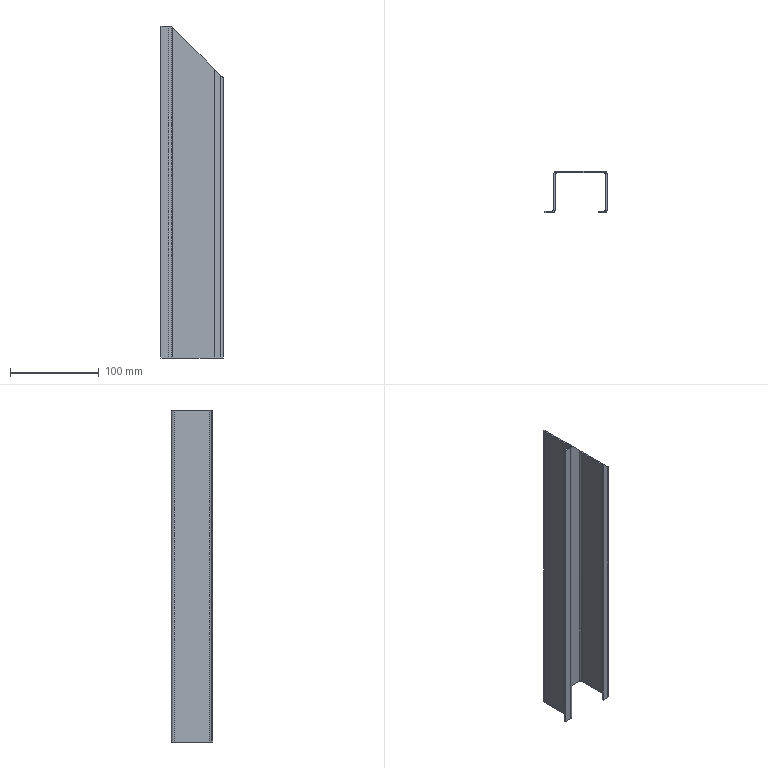Part | STEP file | 750078417 | 1 solid | 28 faces | box 70 x 46.5 x 374 mm | volume 85341 mm3 | plane 17 | cylinder 8 | spline 3 | commonest cylinder face diameters 3 x4 6 x4
STEP:
#1=CARTESIAN_POINT('',(-14.5,45.,318.5));
#2=VERTEX_POINT('',#1);
#3=CARTESIAN_POINT('',(-14.5,45.,0.));
#4=VERTEX_POINT('',#3);
#5=CARTESIAN_POINT('',(-14.5,45.,0.));
#6=DIRECTION('',(0.,0.,-1.));
#7=VECTOR('',#6,1000.);
#8=LINE('',#5,#7);
#9=EDGE_CURVE('',#2,#4,#8,.T.);
#10=ORIENTED_EDGE('',*,*,#9,.T.);
#11=CARTESIAN_POINT('',(-68.5,45.,0.));
#12=VERTEX_POINT('',#11);
#13=CARTESIAN_POINT('',(-11.5,45.,0.));
#14=DIRECTION('',(-1.,0.,0.));
#15=VECTOR('',#14,1000.);
#16=LINE('',#13,#15);
#17=EDGE_CURVE('',#4,#12,#16,.T.);
#18=ORIENTED_EDGE('',*,*,#17,.T.);
#19=CARTESIAN_POINT('',(-68.5,45.,372.5));
#20=VERTEX_POINT('',#19);
#21=CARTESIAN_POINT('',(-68.5,45.,0.));
#22=DIRECTION('',(0.,0.,1.));
#23=VECTOR('',#22,1000.);
#24=LINE('',#21,#23);
#25=EDGE_CURVE('',#12,#20,#24,.T.);
#26=ORIENTED_EDGE('',*,*,#25,.T.);
#27=CARTESIAN_POINT('',(-68.5,45.,372.5));
#28=DIRECTION('',(0.7071,0.,-0.7071));
#29=VECTOR('',#28,1000.);
#30=LINE('',#27,#29);
#31=EDGE_CURVE('',#20,#2,#30,.T.);
#32=ORIENTED_EDGE('',*,*,#31,.T.);
#33=EDGE_LOOP('',(#10,#18,#26,#32));
#34=FACE_OUTER_BOUND('',#33,.T.);
#35=CARTESIAN_POINT('',(-11.5,45.,0.));
#36=DIRECTION('',(0.,1.,0.));
#37=DIRECTION('',(-1.,0.,0.));
#38=AXIS2_PLACEMENT_3D('',#35,#36,#37);
#39=PLANE('',#38);
#40=ADVANCED_FACE('',(#34),#39,.T.);
#41=CARTESIAN_POINT('',(-14.5,-1.5,0.));
#42=VERTEX_POINT('',#41);
#43=CARTESIAN_POINT('',(-21.5,-1.5,0.));
#44=VERTEX_POINT('',#43);
#45=CARTESIAN_POINT('',(-21.5,-1.5,0.));
#46=DIRECTION('',(-1.,0.,0.));
#47=VECTOR('',#46,1000.);
#48=LINE('',#45,#47);
#49=EDGE_CURVE('',#42,#44,#48,.T.);
#50=ORIENTED_EDGE('',*,*,#49,.T.);
#51=CARTESIAN_POINT('',(-21.5,0.,0.));
#52=VERTEX_POINT('',#51);
#53=CARTESIAN_POINT('',(-21.5,-1.5,0.));
#54=DIRECTION('',(0.,1.,0.));
#55=VECTOR('',#54,1000.);
#56=LINE('',#53,#55);
#57=EDGE_CURVE('',#44,#52,#56,.T.);
#58=ORIENTED_EDGE('',*,*,#57,.T.);
#59=CARTESIAN_POINT('',(-14.5,0.,0.));
#60=VERTEX_POINT('',#59);
#61=CARTESIAN_POINT('',(-21.5,0.,0.));
#62=DIRECTION('',(1.,0.,0.));
#63=VECTOR('',#62,1000.);
#64=LINE('',#61,#63);
#65=EDGE_CURVE('',#52,#60,#64,.T.);
#66=ORIENTED_EDGE('',*,*,#65,.T.);
#67=CARTESIAN_POINT('',(-13.,1.5,0.));
#68=VERTEX_POINT('',#67);
#69=CARTESIAN_POINT('',(-14.5,1.5,0.));
#70=DIRECTION('',(0.,0.,1.));
#71=DIRECTION('',(1.,0.,0.));
#72=AXIS2_PLACEMENT_3D('',#69,#70,#71);
#73=CIRCLE('',#72,1.5);
#74=EDGE_CURVE('',#60,#68,#73,.T.);
#75=ORIENTED_EDGE('',*,*,#74,.T.);
#76=CARTESIAN_POINT('',(-13.,42.,0.));
#77=VERTEX_POINT('',#76);
#78=CARTESIAN_POINT('',(-13.,-1.5,0.));
#79=DIRECTION('',(0.,1.,0.));
#80=VECTOR('',#79,1000.);
#81=LINE('',#78,#80);
#82=EDGE_CURVE('',#68,#77,#81,.T.);
#83=ORIENTED_EDGE('',*,*,#82,.T.);
#84=CARTESIAN_POINT('',(-14.5,43.5,0.));
#85=VERTEX_POINT('',#84);
#86=CARTESIAN_POINT('',(-14.5,42.,0.));
#87=DIRECTION('',(0.,0.,1.));
#88=DIRECTION('',(1.,0.,0.));
#89=AXIS2_PLACEMENT_3D('',#86,#87,#88);
#90=CIRCLE('',#89,1.5);
#91=EDGE_CURVE('',#77,#85,#90,.T.);
#92=ORIENTED_EDGE('',*,*,#91,.T.);
#93=CARTESIAN_POINT('',(-68.5,43.5,0.));
#94=VERTEX_POINT('',#93);
#95=CARTESIAN_POINT('',(-21.5,43.5,0.));
#96=DIRECTION('',(-1.,0.,0.));
#97=VECTOR('',#96,1000.);
#98=LINE('',#95,#97);
#99=EDGE_CURVE('',#85,#94,#98,.T.);
#100=ORIENTED_EDGE('',*,*,#99,.T.);
#101=CARTESIAN_POINT('',(-70.,42.,0.));
#102=VERTEX_POINT('',#101);
#103=CARTESIAN_POINT('',(-68.5,42.,0.));
#104=DIRECTION('',(0.,0.,1.));
#105=DIRECTION('',(1.,0.,0.));
#106=AXIS2_PLACEMENT_3D('',#103,#104,#105);
#107=CIRCLE('',#106,1.5);
#108=EDGE_CURVE('',#94,#102,#107,.T.);
#109=ORIENTED_EDGE('',*,*,#108,.T.);
#110=CARTESIAN_POINT('',(-70.,1.5,0.));
#111=VERTEX_POINT('',#110);
#112=CARTESIAN_POINT('',(-70.,-1.5,0.));
#113=DIRECTION('',(0.,-1.,0.));
#114=VECTOR('',#113,1000.);
#115=LINE('',#112,#114);
#116=EDGE_CURVE('',#102,#111,#115,.T.);
#117=ORIENTED_EDGE('',*,*,#116,.T.);
#118=CARTESIAN_POINT('',(-73.,-1.5,0.));
#119=VERTEX_POINT('',#118);
#120=CARTESIAN_POINT('',(-73.,1.5,0.));
#121=DIRECTION('',(0.,0.,-1.));
#122=DIRECTION('',(1.,0.,0.));
#123=AXIS2_PLACEMENT_3D('',#120,#121,#122);
#124=CIRCLE('',#123,3.);
#125=EDGE_CURVE('',#111,#119,#124,.T.);
#126=ORIENTED_EDGE('',*,*,#125,.T.);
#127=CARTESIAN_POINT('',(-81.5,-1.5,0.));
#128=VERTEX_POINT('',#127);
#129=CARTESIAN_POINT('',(-21.5,-1.5,0.));
#130=DIRECTION('',(-1.,0.,0.));
#131=VECTOR('',#130,1000.);
#132=LINE('',#129,#131);
#133=EDGE_CURVE('',#119,#128,#132,.T.);
#134=ORIENTED_EDGE('',*,*,#133,.T.);
#135=CARTESIAN_POINT('',(-81.5,0.,0.));
#136=VERTEX_POINT('',#135);
#137=CARTESIAN_POINT('',(-81.5,0.,0.));
#138=DIRECTION('',(0.,-1.,0.));
#139=VECTOR('',#138,1000.);
#140=LINE('',#137,#139);
#141=EDGE_CURVE('',#136,#128,#140,.T.);
#142=ORIENTED_EDGE('',*,*,#141,.F.);
#143=CARTESIAN_POINT('',(-73.,0.,0.));
#144=VERTEX_POINT('',#143);
#145=CARTESIAN_POINT('',(-21.5,0.,0.));
#146=DIRECTION('',(1.,0.,0.));
#147=VECTOR('',#146,1000.);
#148=LINE('',#145,#147);
#149=EDGE_CURVE('',#136,#144,#148,.T.);
#150=ORIENTED_EDGE('',*,*,#149,.T.);
#151=CARTESIAN_POINT('',(-71.5,1.5,0.));
#152=VERTEX_POINT('',#151);
#153=CARTESIAN_POINT('',(-73.,1.5,0.));
#154=DIRECTION('',(0.,0.,1.));
#155=DIRECTION('',(1.,0.,0.));
#156=AXIS2_PLACEMENT_3D('',#153,#154,#155);
#157=CIRCLE('',#156,1.5);
#158=EDGE_CURVE('',#144,#152,#157,.T.);
#159=ORIENTED_EDGE('',*,*,#158,.T.);
#160=CARTESIAN_POINT('',(-71.5,42.,0.));
#161=VERTEX_POINT('',#160);
#162=CARTESIAN_POINT('',(-71.5,-1.5,0.));
#163=DIRECTION('',(0.,1.,0.));
#164=VECTOR('',#163,1000.);
#165=LINE('',#162,#164);
#166=EDGE_CURVE('',#152,#161,#165,.T.);
#167=ORIENTED_EDGE('',*,*,#166,.T.);
#168=CARTESIAN_POINT('',(-68.5,42.,0.));
#169=DIRECTION('',(0.,0.,-1.));
#170=DIRECTION('',(1.,0.,0.));
#171=AXIS2_PLACEMENT_3D('',#168,#169,#170);
#172=CIRCLE('',#171,3.);
#173=EDGE_CURVE('',#161,#12,#172,.T.);
#174=ORIENTED_EDGE('',*,*,#173,.T.);
#175=ORIENTED_EDGE('',*,*,#17,.F.);
#176=CARTESIAN_POINT('',(-11.5,42.,0.));
#177=VERTEX_POINT('',#176);
#178=CARTESIAN_POINT('',(-14.5,42.,0.));
#179=DIRECTION('',(0.,0.,-1.));
#180=DIRECTION('',(1.,0.,0.));
#181=AXIS2_PLACEMENT_3D('',#178,#179,#180);
#182=CIRCLE('',#181,3.);
#183=EDGE_CURVE('',#4,#177,#182,.T.);
#184=ORIENTED_EDGE('',*,*,#183,.T.);
#185=CARTESIAN_POINT('',(-11.5,1.5,0.));
#186=VERTEX_POINT('',#185);
#187=CARTESIAN_POINT('',(-11.5,-1.5,0.));
#188=DIRECTION('',(0.,-1.,0.));
#189=VECTOR('',#188,1000.);
#190=LINE('',#187,#189);
#191=EDGE_CURVE('',#177,#186,#190,.T.);
#192=ORIENTED_EDGE('',*,*,#191,.T.);
#193=CARTESIAN_POINT('',(-14.5,1.5,0.));
#194=DIRECTION('',(0.,0.,-1.));
#195=DIRECTION('',(1.,0.,0.));
#196=AXIS2_PLACEMENT_3D('',#193,#194,#195);
#197=CIRCLE('',#196,3.);
#198=EDGE_CURVE('',#186,#42,#197,.T.);
#199=ORIENTED_EDGE('',*,*,#198,.T.);
#200=EDGE_LOOP('',(#50,#58,#66,#75,#83,#92,#100,#109,#117,#126,#134,#142,#150,#159,#167,#174,#175,#184,#192,#199));
#201=FACE_OUTER_BOUND('',#200,.T.);
#202=CARTESIAN_POINT('',(-21.5,-1.5,0.));
#203=DIRECTION('',(0.,0.,-1.));
#204=DIRECTION('',(-1.,0.,0.));
#205=AXIS2_PLACEMENT_3D('',#202,#203,#204);
#206=PLANE('',#205);
#207=ADVANCED_FACE('',(#201),#206,.T.);
#208=CARTESIAN_POINT('',(-11.5,42.,315.5));
#209=VERTEX_POINT('',#208);
#210=CARTESIAN_POINT('',(-11.5,42.,0.));
#211=DIRECTION('',(0.,0.,-1.));
#212=VECTOR('',#211,1000.);
#213=LINE('',#210,#212);
#214=EDGE_CURVE('',#209,#177,#213,.T.);
#215=ORIENTED_EDGE('',*,*,#214,.T.);
#216=ORIENTED_EDGE('',*,*,#183,.F.);
#217=ORIENTED_EDGE('',*,*,#9,.F.);
#218=CARTESIAN_POINT('',(-14.5,45.,318.5));
#219=CARTESIAN_POINT('',(-12.5,45.,316.5));
#220=CARTESIAN_POINT('',(-11.5,43.5,315.5));
#221=CARTESIAN_POINT('',(-11.5,42.,315.5));
#222=(BOUNDED_CURVE()B_SPLINE_CURVE(3,(#218,#219,#220,#221),.UNSPECIFIED.,.F.,.T.)B_SPLINE_CURVE_WITH_KNOTS((4,4),(0.,0.005675),.UNSPECIFIED.)CURVE()GEOMETRIC_REPRESENTATION_ITEM()RATIONAL_B_SPLINE_CURVE((0.5,0.5,0.6667,1.))REPRESENTATION_ITEM(''));
#223=EDGE_CURVE('',#2,#209,#222,.T.);
#224=ORIENTED_EDGE('',*,*,#223,.T.);
#225=EDGE_LOOP('',(#215,#216,#217,#224));
#226=FACE_OUTER_BOUND('',#225,.T.);
#227=CARTESIAN_POINT('',(-14.5,42.,0.));
#228=DIRECTION('',(0.,0.,1.));
#229=DIRECTION('',(1.,0.,0.));
#230=AXIS2_PLACEMENT_3D('',#227,#228,#229);
#231=CYLINDRICAL_SURFACE('',#230,3.);
#232=ADVANCED_FACE('',(#226),#231,.T.);
#233=CARTESIAN_POINT('',(-68.5,43.5,372.5));
#234=VERTEX_POINT('',#233);
#235=CARTESIAN_POINT('',(-68.5,44.25,372.5));
#236=DIRECTION('',(0.,-1.,0.));
#237=VECTOR('',#236,1000.);
#238=LINE('',#235,#237);
#239=EDGE_CURVE('',#20,#234,#238,.T.);
#240=ORIENTED_EDGE('',*,*,#239,.T.);
#241=CARTESIAN_POINT('',(-14.5,43.5,318.5));
#242=VERTEX_POINT('',#241);
#243=CARTESIAN_POINT('',(146.25,43.5,157.75));
#244=DIRECTION('',(0.7071,0.,-0.7071));
#245=VECTOR('',#244,1000.);
#246=LINE('',#243,#245);
#247=EDGE_CURVE('',#234,#242,#246,.T.);
#248=ORIENTED_EDGE('',*,*,#247,.T.);
#249=CARTESIAN_POINT('',(-14.5,45.,318.5));
#250=DIRECTION('',(0.,1.,0.));
#251=VECTOR('',#250,1000.);
#252=LINE('',#249,#251);
#253=EDGE_CURVE('',#242,#2,#252,.T.);
#254=ORIENTED_EDGE('',*,*,#253,.T.);
#255=ORIENTED_EDGE('',*,*,#31,.F.);
#256=EDGE_LOOP('',(#240,#248,#254,#255));
#257=FACE_OUTER_BOUND('',#256,.T.);
#258=CARTESIAN_POINT('',(146.25,45.,157.75));
#259=DIRECTION('',(0.7071,0.,0.7071));
#260=DIRECTION('',(0.7071,0.,-0.7071));
#261=AXIS2_PLACEMENT_3D('',#258,#259,#260);
#262=PLANE('',#261);
#263=ADVANCED_FACE('',(#257),#262,.T.);
#264=ORIENTED_EDGE('',*,*,#25,.F.);
#265=ORIENTED_EDGE('',*,*,#173,.F.);
#266=CARTESIAN_POINT('',(-71.5,42.,374.));
#267=VERTEX_POINT('',#266);
#268=CARTESIAN_POINT('',(-71.5,42.,0.));
#269=DIRECTION('',(0.,0.,1.));
#270=VECTOR('',#269,1000.);
#271=LINE('',#268,#270);
#272=EDGE_CURVE('',#161,#267,#271,.T.);
#273=ORIENTED_EDGE('',*,*,#272,.T.);
#274=CARTESIAN_POINT('',(-71.5,42.,374.));
#275=CARTESIAN_POINT('',(-71.5,43.5,374.));
#276=CARTESIAN_POINT('',(-70.5,45.,373.5));
#277=CARTESIAN_POINT('',(-68.5,45.,372.5));
#278=(BOUNDED_CURVE()B_SPLINE_CURVE(3,(#274,#275,#276,#277),.UNSPECIFIED.,.F.,.F.)B_SPLINE_CURVE_WITH_KNOTS((4,4),(0.,0.00497),.UNSPECIFIED.)CURVE()GEOMETRIC_REPRESENTATION_ITEM()RATIONAL_B_SPLINE_CURVE((1.,0.6667,0.5,0.5))REPRESENTATION_ITEM(''));
#279=EDGE_CURVE('',#267,#20,#278,.T.);
#280=ORIENTED_EDGE('',*,*,#279,.T.);
#281=EDGE_LOOP('',(#264,#265,#273,#280));
#282=FACE_OUTER_BOUND('',#281,.T.);
#283=CARTESIAN_POINT('',(-68.5,42.,0.));
#284=DIRECTION('',(0.,0.,1.));
#285=DIRECTION('',(1.,0.,0.));
#286=AXIS2_PLACEMENT_3D('',#283,#284,#285);
#287=CYLINDRICAL_SURFACE('',#286,3.);
#288=ADVANCED_FACE('',(#282),#287,.T.);
#289=CARTESIAN_POINT('',(-21.5,-1.5,325.5));
#290=VERTEX_POINT('',#289);
#291=CARTESIAN_POINT('',(-21.5,-1.5,0.));
#292=DIRECTION('',(0.,0.,-1.));
#293=VECTOR('',#292,1000.);
#294=LINE('',#291,#293);
#295=EDGE_CURVE('',#290,#44,#294,.T.);
#296=ORIENTED_EDGE('',*,*,#295,.T.);
#297=ORIENTED_EDGE('',*,*,#49,.F.);
#298=CARTESIAN_POINT('',(-14.5,-1.5,318.5));
#299=VERTEX_POINT('',#298);
#300=CARTESIAN_POINT('',(-14.5,-1.5,0.));
#301=DIRECTION('',(0.,0.,1.));
#302=VECTOR('',#301,1000.);
#303=LINE('',#300,#302);
#304=EDGE_CURVE('',#42,#299,#303,.T.);
#305=ORIENTED_EDGE('',*,*,#304,.T.);
#306=CARTESIAN_POINT('',(-14.5,-1.5,318.5));
#307=DIRECTION('',(-0.7071,0.,0.7071));
#308=VECTOR('',#307,1000.);
#309=LINE('',#306,#308);
#310=EDGE_CURVE('',#299,#290,#309,.T.);
#311=ORIENTED_EDGE('',*,*,#310,.T.);
#312=EDGE_LOOP('',(#296,#297,#305,#311));
#313=FACE_OUTER_BOUND('',#312,.T.);
#314=CARTESIAN_POINT('',(-21.5,-1.5,0.));
#315=DIRECTION('',(0.,-1.,0.));
#316=DIRECTION('',(1.,0.,0.));
#317=AXIS2_PLACEMENT_3D('',#314,#315,#316);
#318=PLANE('',#317);
#319=ADVANCED_FACE('',(#313),#318,.T.);
#320=ORIENTED_EDGE('',*,*,#304,.F.);
#321=ORIENTED_EDGE('',*,*,#198,.F.);
#322=CARTESIAN_POINT('',(-11.5,1.5,315.5));
#323=VERTEX_POINT('',#322);
#324=CARTESIAN_POINT('',(-11.5,1.5,0.));
#325=DIRECTION('',(0.,0.,1.));
#326=VECTOR('',#325,1000.);
#327=LINE('',#324,#326);
#328=EDGE_CURVE('',#186,#323,#327,.T.);
#329=ORIENTED_EDGE('',*,*,#328,.T.);
#330=CARTESIAN_POINT('',(-11.5,1.5,315.5));
#331=CARTESIAN_POINT('',(-11.5,0.,315.5));
#332=CARTESIAN_POINT('',(-12.5,-1.5,316.5));
#333=CARTESIAN_POINT('',(-14.5,-1.5,318.5));
#334=(BOUNDED_CURVE()B_SPLINE_CURVE(3,(#330,#331,#332,#333),.UNSPECIFIED.,.F.,.F.)B_SPLINE_CURVE_WITH_KNOTS((4,4),(0.,0.005784),.UNSPECIFIED.)CURVE()GEOMETRIC_REPRESENTATION_ITEM()RATIONAL_B_SPLINE_CURVE((1.,0.6667,0.5,0.5))REPRESENTATION_ITEM(''));
#335=EDGE_CURVE('',#323,#299,#334,.T.);
#336=ORIENTED_EDGE('',*,*,#335,.T.);
#337=EDGE_LOOP('',(#320,#321,#329,#336));
#338=FACE_OUTER_BOUND('',#337,.T.);
#339=CARTESIAN_POINT('',(-14.5,1.5,0.));
#340=DIRECTION('',(0.,0.,1.));
#341=DIRECTION('',(1.,0.,0.));
#342=AXIS2_PLACEMENT_3D('',#339,#340,#341);
#343=CYLINDRICAL_SURFACE('',#342,3.);
#344=ADVANCED_FACE('',(#338),#343,.T.);
#345=ORIENTED_EDGE('',*,*,#328,.F.);
#346=ORIENTED_EDGE('',*,*,#191,.F.);
#347=ORIENTED_EDGE('',*,*,#214,.F.);
#348=CARTESIAN_POINT('',(-11.5,-1.5,315.5));
#349=DIRECTION('',(0.,-1.,0.));
#350=VECTOR('',#349,1000.);
#351=LINE('',#348,#350);
#352=EDGE_CURVE('',#209,#323,#351,.T.);
#353=ORIENTED_EDGE('',*,*,#352,.T.);
#354=EDGE_LOOP('',(#345,#346,#347,#353));
#355=FACE_OUTER_BOUND('',#354,.T.);
#356=CARTESIAN_POINT('',(-11.5,-1.5,0.));
#357=DIRECTION('',(1.,0.,0.));
#358=DIRECTION('',(0.,0.,-1.));
#359=AXIS2_PLACEMENT_3D('',#356,#357,#358);
#360=PLANE('',#359);
#361=ADVANCED_FACE('',(#355),#360,.T.);
#362=ORIENTED_EDGE('',*,*,#166,.F.);
#363=CARTESIAN_POINT('',(-71.5,1.5,374.));
#364=VERTEX_POINT('',#363);
#365=CARTESIAN_POINT('',(-71.5,1.5,0.));
#366=DIRECTION('',(0.,0.,1.));
#367=VECTOR('',#366,1000.);
#368=LINE('',#365,#367);
#369=EDGE_CURVE('',#152,#364,#368,.T.);
#370=ORIENTED_EDGE('',*,*,#369,.T.);
#371=CARTESIAN_POINT('',(-71.5,45.,374.));
#372=DIRECTION('',(0.,1.,0.));
#373=VECTOR('',#372,1000.);
#374=LINE('',#371,#373);
#375=EDGE_CURVE('',#364,#267,#374,.T.);
#376=ORIENTED_EDGE('',*,*,#375,.T.);
#377=ORIENTED_EDGE('',*,*,#272,.F.);
#378=EDGE_LOOP('',(#362,#370,#376,#377));
#379=FACE_OUTER_BOUND('',#378,.T.);
#380=CARTESIAN_POINT('',(-71.5,45.,0.));
#381=DIRECTION('',(-1.,0.,0.));
#382=DIRECTION('',(0.,0.,1.));
#383=AXIS2_PLACEMENT_3D('',#380,#381,#382);
#384=PLANE('',#383);
#385=ADVANCED_FACE('',(#379),#384,.T.);
#386=ORIENTED_EDGE('',*,*,#369,.F.);
#387=ORIENTED_EDGE('',*,*,#158,.F.);
#388=CARTESIAN_POINT('',(-73.,0.,374.));
#389=VERTEX_POINT('',#388);
#390=CARTESIAN_POINT('',(-73.,0.,0.));
#391=DIRECTION('',(0.,0.,-1.));
#392=VECTOR('',#391,1000.);
#393=LINE('',#390,#392);
#394=EDGE_CURVE('',#389,#144,#393,.T.);
#395=ORIENTED_EDGE('',*,*,#394,.F.);
#396=CARTESIAN_POINT('',(-73.,1.5,374.));
#397=DIRECTION('',(0.,0.,-1.));
#398=DIRECTION('',(1.,0.,0.));
#399=AXIS2_PLACEMENT_3D('',#396,#397,#398);
#400=CIRCLE('',#399,1.5);
#401=EDGE_CURVE('',#364,#389,#400,.T.);
#402=ORIENTED_EDGE('',*,*,#401,.F.);
#403=EDGE_LOOP('',(#386,#387,#395,#402));
#404=FACE_OUTER_BOUND('',#403,.T.);
#405=CARTESIAN_POINT('',(-73.,1.5,0.));
#406=DIRECTION('',(0.,0.,1.));
#407=DIRECTION('',(1.,0.,0.));
#408=AXIS2_PLACEMENT_3D('',#405,#406,#407);
#409=CYLINDRICAL_SURFACE('',#408,1.5);
#410=ADVANCED_FACE('',(#404),#409,.F.);
#411=ORIENTED_EDGE('',*,*,#149,.F.);
#412=CARTESIAN_POINT('',(-81.5,0.,374.));
#413=VERTEX_POINT('',#412);
#414=CARTESIAN_POINT('',(-81.5,0.,0.));
#415=DIRECTION('',(0.,0.,1.));
#416=VECTOR('',#415,1000.);
#417=LINE('',#414,#416);
#418=EDGE_CURVE('',#136,#413,#417,.T.);
#419=ORIENTED_EDGE('',*,*,#418,.T.);
#420=CARTESIAN_POINT('',(-71.5,0.,374.));
#421=DIRECTION('',(1.,0.,0.));
#422=VECTOR('',#421,1000.);
#423=LINE('',#420,#422);
#424=EDGE_CURVE('',#413,#389,#423,.T.);
#425=ORIENTED_EDGE('',*,*,#424,.T.);
#426=ORIENTED_EDGE('',*,*,#394,.T.);
#427=EDGE_LOOP('',(#411,#419,#425,#426));
#428=FACE_OUTER_BOUND('',#427,.T.);
#429=CARTESIAN_POINT('',(-71.5,0.,0.));
#430=DIRECTION('',(0.,1.,0.));
#431=DIRECTION('',(-1.,0.,0.));
#432=AXIS2_PLACEMENT_3D('',#429,#430,#431);
#433=PLANE('',#432);
#434=ADVANCED_FACE('',(#428),#433,.T.);
#435=CARTESIAN_POINT('',(-81.5,-1.5,374.));
#436=VERTEX_POINT('',#435);
#437=CARTESIAN_POINT('',(-81.5,-1.5,0.));
#438=DIRECTION('',(0.,0.,1.));
#439=VECTOR('',#438,1000.);
#440=LINE('',#437,#439);
#441=EDGE_CURVE('',#128,#436,#440,.T.);
#442=ORIENTED_EDGE('',*,*,#441,.F.);
#443=ORIENTED_EDGE('',*,*,#133,.F.);
#444=CARTESIAN_POINT('',(-73.,-1.5,374.));
#445=VERTEX_POINT('',#444);
#446=CARTESIAN_POINT('',(-73.,-1.5,0.));
#447=DIRECTION('',(0.,0.,-1.));
#448=VECTOR('',#447,1000.);
#449=LINE('',#446,#448);
#450=EDGE_CURVE('',#445,#119,#449,.T.);
#451=ORIENTED_EDGE('',*,*,#450,.F.);
#452=CARTESIAN_POINT('',(-71.5,-1.5,374.));
#453=DIRECTION('',(1.,0.,0.));
#454=VECTOR('',#453,1000.);
#455=LINE('',#452,#454);
#456=EDGE_CURVE('',#436,#445,#455,.T.);
#457=ORIENTED_EDGE('',*,*,#456,.F.);
#458=EDGE_LOOP('',(#442,#443,#451,#457));
#459=FACE_OUTER_BOUND('',#458,.T.);
#460=CARTESIAN_POINT('',(-71.5,-1.5,0.));
#461=DIRECTION('',(0.,1.,0.));
#462=DIRECTION('',(-1.,0.,0.));
#463=AXIS2_PLACEMENT_3D('',#460,#461,#462);
#464=PLANE('',#463);
#465=ADVANCED_FACE('',(#459),#464,.F.);
#466=ORIENTED_EDGE('',*,*,#125,.F.);
#467=CARTESIAN_POINT('',(-70.,1.5,374.));
#468=VERTEX_POINT('',#467);
#469=CARTESIAN_POINT('',(-70.,1.5,0.));
#470=DIRECTION('',(0.,0.,1.));
#471=VECTOR('',#470,1000.);
#472=LINE('',#469,#471);
#473=EDGE_CURVE('',#111,#468,#472,.T.);
#474=ORIENTED_EDGE('',*,*,#473,.T.);
#475=CARTESIAN_POINT('',(-73.,1.5,374.));
#476=DIRECTION('',(0.,0.,-1.));
#477=DIRECTION('',(1.,0.,0.));
#478=AXIS2_PLACEMENT_3D('',#475,#476,#477);
#479=CIRCLE('',#478,3.);
#480=EDGE_CURVE('',#468,#445,#479,.T.);
#481=ORIENTED_EDGE('',*,*,#480,.T.);
#482=ORIENTED_EDGE('',*,*,#450,.T.);
#483=EDGE_LOOP('',(#466,#474,#481,#482));
#484=FACE_OUTER_BOUND('',#483,.T.);
#485=CARTESIAN_POINT('',(-73.,1.5,0.));
#486=DIRECTION('',(0.,0.,1.));
#487=DIRECTION('',(1.,0.,0.));
#488=AXIS2_PLACEMENT_3D('',#485,#486,#487);
#489=CYLINDRICAL_SURFACE('',#488,3.);
#490=ADVANCED_FACE('',(#484),#489,.T.);
#491=ORIENTED_EDGE('',*,*,#473,.F.);
#492=ORIENTED_EDGE('',*,*,#116,.F.);
#493=CARTESIAN_POINT('',(-70.,42.,374.));
#494=VERTEX_POINT('',#493);
#495=CARTESIAN_POINT('',(-70.,42.,0.));
#496=DIRECTION('',(0.,0.,-1.));
#497=VECTOR('',#496,1000.);
#498=LINE('',#495,#497);
#499=EDGE_CURVE('',#494,#102,#498,.T.);
#500=ORIENTED_EDGE('',*,*,#499,.F.);
#501=CARTESIAN_POINT('',(-70.,45.,374.));
#502=DIRECTION('',(0.,1.,0.));
#503=VECTOR('',#502,1000.);
#504=LINE('',#501,#503);
#505=EDGE_CURVE('',#468,#494,#504,.T.);
#506=ORIENTED_EDGE('',*,*,#505,.F.);
#507=EDGE_LOOP('',(#491,#492,#500,#506));
#508=FACE_OUTER_BOUND('',#507,.T.);
#509=CARTESIAN_POINT('',(-70.,45.,0.));
#510=DIRECTION('',(-1.,0.,0.));
#511=DIRECTION('',(0.,0.,1.));
#512=AXIS2_PLACEMENT_3D('',#509,#510,#511);
#513=PLANE('',#512);
#514=ADVANCED_FACE('',(#508),#513,.F.);
#515=ORIENTED_EDGE('',*,*,#499,.T.);
#516=ORIENTED_EDGE('',*,*,#108,.F.);
#517=CARTESIAN_POINT('',(-68.5,43.5,0.));
#518=DIRECTION('',(0.,0.,-1.));
#519=VECTOR('',#518,1000.);
#520=LINE('',#517,#519);
#521=EDGE_CURVE('',#234,#94,#520,.T.);
#522=ORIENTED_EDGE('',*,*,#521,.F.);
#523=CARTESIAN_POINT('',(-70.,42.,374.));
#524=CARTESIAN_POINT('',(-70.,42.75,374.));
#525=CARTESIAN_POINT('',(-69.5,43.5,373.5));
#526=CARTESIAN_POINT('',(-68.5,43.5,372.5));
#527=(BOUNDED_CURVE()B_SPLINE_CURVE(3,(#523,#524,#525,#526),.UNSPECIFIED.,.F.,.F.)B_SPLINE_CURVE_WITH_KNOTS((4,4),(0.,0.002854),.UNSPECIFIED.)CURVE()GEOMETRIC_REPRESENTATION_ITEM()RATIONAL_B_SPLINE_CURVE((1.,0.6667,0.5,0.5))REPRESENTATION_ITEM(''));
#528=EDGE_CURVE('',#494,#234,#527,.T.);
#529=ORIENTED_EDGE('',*,*,#528,.F.);
#530=EDGE_LOOP('',(#515,#516,#522,#529));
#531=FACE_OUTER_BOUND('',#530,.T.);
#532=CARTESIAN_POINT('',(-68.5,42.,0.));
#533=DIRECTION('',(0.,0.,1.));
#534=DIRECTION('',(1.,0.,0.));
#535=AXIS2_PLACEMENT_3D('',#532,#533,#534);
#536=CYLINDRICAL_SURFACE('',#535,1.5);
#537=ADVANCED_FACE('',(#531),#536,.F.);
#538=ORIENTED_EDGE('',*,*,#521,.T.);
#539=ORIENTED_EDGE('',*,*,#99,.F.);
#540=CARTESIAN_POINT('',(-14.5,43.5,0.));
#541=DIRECTION('',(0.,0.,-1.));
#542=VECTOR('',#541,1000.);
#543=LINE('',#540,#542);
#544=EDGE_CURVE('',#242,#85,#543,.T.);
#545=ORIENTED_EDGE('',*,*,#544,.F.);
#546=ORIENTED_EDGE('',*,*,#247,.F.);
#547=EDGE_LOOP('',(#538,#539,#545,#546));
#548=FACE_OUTER_BOUND('',#547,.T.);
#549=CARTESIAN_POINT('',(-11.5,43.5,0.));
#550=DIRECTION('',(0.,1.,0.));
#551=DIRECTION('',(-1.,0.,0.));
#552=AXIS2_PLACEMENT_3D('',#549,#550,#551);
#553=PLANE('',#552);
#554=ADVANCED_FACE('',(#548),#553,.F.);
#555=ORIENTED_EDGE('',*,*,#544,.T.);
#556=ORIENTED_EDGE('',*,*,#91,.F.);
#557=CARTESIAN_POINT('',(-13.,42.,315.5));
#558=VERTEX_POINT('',#557);
#559=CARTESIAN_POINT('',(-13.,42.,0.));
#560=DIRECTION('',(0.,0.,-1.));
#561=VECTOR('',#560,1000.);
#562=LINE('',#559,#561);
#563=EDGE_CURVE('',#558,#77,#562,.T.);
#564=ORIENTED_EDGE('',*,*,#563,.F.);
#565=CARTESIAN_POINT('',(-14.5,43.5,318.5));
#566=CARTESIAN_POINT('',(-13.5,43.5,316.5));
#567=CARTESIAN_POINT('',(-13.,42.75,315.5));
#568=CARTESIAN_POINT('',(-13.,42.,315.5));
#569=(BOUNDED_CURVE()B_SPLINE_CURVE(3,(#565,#566,#567,#568),.UNSPECIFIED.,.F.,.F.)B_SPLINE_CURVE_WITH_KNOTS((4,4),(0.,0.003921),.UNSPECIFIED.)CURVE()GEOMETRIC_REPRESENTATION_ITEM()RATIONAL_B_SPLINE_CURVE((0.5,0.5,0.6667,1.))REPRESENTATION_ITEM(''));
#570=EDGE_CURVE('',#242,#558,#569,.T.);
#571=ORIENTED_EDGE('',*,*,#570,.F.);
#572=EDGE_LOOP('',(#555,#556,#564,#571));
#573=FACE_OUTER_BOUND('',#572,.T.);
#574=CARTESIAN_POINT('',(-14.5,42.,0.));
#575=DIRECTION('',(0.,0.,1.));
#576=DIRECTION('',(1.,0.,0.));
#577=AXIS2_PLACEMENT_3D('',#574,#575,#576);
#578=CYLINDRICAL_SURFACE('',#577,1.5);
#579=ADVANCED_FACE('',(#573),#578,.F.);
#580=ORIENTED_EDGE('',*,*,#563,.T.);
#581=ORIENTED_EDGE('',*,*,#82,.F.);
#582=CARTESIAN_POINT('',(-13.,1.5,315.5));
#583=VERTEX_POINT('',#582);
#584=CARTESIAN_POINT('',(-13.,1.5,0.));
#585=DIRECTION('',(0.,0.,-1.));
#586=VECTOR('',#585,1000.);
#587=LINE('',#584,#586);
#588=EDGE_CURVE('',#583,#68,#587,.T.);
#589=ORIENTED_EDGE('',*,*,#588,.F.);
#590=CARTESIAN_POINT('',(-13.,-1.5,315.5));
#591=DIRECTION('',(0.,-1.,0.));
#592=VECTOR('',#591,1000.);
#593=LINE('',#590,#592);
#594=EDGE_CURVE('',#558,#583,#593,.T.);
#595=ORIENTED_EDGE('',*,*,#594,.F.);
#596=EDGE_LOOP('',(#580,#581,#589,#595));
#597=FACE_OUTER_BOUND('',#596,.T.);
#598=CARTESIAN_POINT('',(-13.,-1.5,0.));
#599=DIRECTION('',(1.,0.,0.));
#600=DIRECTION('',(0.,0.,-1.));
#601=AXIS2_PLACEMENT_3D('',#598,#599,#600);
#602=PLANE('',#601);
#603=ADVANCED_FACE('',(#597),#602,.F.);
#604=ORIENTED_EDGE('',*,*,#588,.T.);
#605=ORIENTED_EDGE('',*,*,#74,.F.);
#606=CARTESIAN_POINT('',(-14.5,0.,318.5));
#607=VERTEX_POINT('',#606);
#608=CARTESIAN_POINT('',(-14.5,0.,0.));
#609=DIRECTION('',(0.,0.,-1.));
#610=VECTOR('',#609,1000.);
#611=LINE('',#608,#610);
#612=EDGE_CURVE('',#607,#60,#611,.T.);
#613=ORIENTED_EDGE('',*,*,#612,.F.);
#614=CARTESIAN_POINT('',(-13.,1.5,315.5));
#615=CARTESIAN_POINT('',(-13.,0.75,315.5));
#616=CARTESIAN_POINT('',(-13.5,0.,316.5));
#617=CARTESIAN_POINT('',(-14.5,0.,318.5));
#618=(BOUNDED_CURVE()B_SPLINE_CURVE(3,(#614,#615,#616,#617),.UNSPECIFIED.,.F.,.F.)B_SPLINE_CURVE_WITH_KNOTS((4,4),(0.,0.003968),.UNSPECIFIED.)CURVE()GEOMETRIC_REPRESENTATION_ITEM()RATIONAL_B_SPLINE_CURVE((1.,0.6667,0.5,0.5))REPRESENTATION_ITEM(''));
#619=EDGE_CURVE('',#583,#607,#618,.T.);
#620=ORIENTED_EDGE('',*,*,#619,.F.);
#621=EDGE_LOOP('',(#604,#605,#613,#620));
#622=FACE_OUTER_BOUND('',#621,.T.);
#623=CARTESIAN_POINT('',(-14.5,1.5,0.));
#624=DIRECTION('',(0.,0.,1.));
#625=DIRECTION('',(1.,0.,0.));
#626=AXIS2_PLACEMENT_3D('',#623,#624,#625);
#627=CYLINDRICAL_SURFACE('',#626,1.5);
#628=ADVANCED_FACE('',(#622),#627,.F.);
#629=ORIENTED_EDGE('',*,*,#612,.T.);
#630=ORIENTED_EDGE('',*,*,#65,.F.);
#631=CARTESIAN_POINT('',(-21.5,0.,325.5));
#632=VERTEX_POINT('',#631);
#633=CARTESIAN_POINT('',(-21.5,0.,0.));
#634=DIRECTION('',(0.,0.,-1.));
#635=VECTOR('',#634,1000.);
#636=LINE('',#633,#635);
#637=EDGE_CURVE('',#632,#52,#636,.T.);
#638=ORIENTED_EDGE('',*,*,#637,.F.);
#639=CARTESIAN_POINT('',(-14.5,0.,318.5));
#640=DIRECTION('',(-0.7071,0.,0.7071));
#641=VECTOR('',#640,1000.);
#642=LINE('',#639,#641);
#643=EDGE_CURVE('',#607,#632,#642,.T.);
#644=ORIENTED_EDGE('',*,*,#643,.F.);
#645=EDGE_LOOP('',(#629,#630,#638,#644));
#646=FACE_OUTER_BOUND('',#645,.T.);
#647=CARTESIAN_POINT('',(-21.5,0.,0.));
#648=DIRECTION('',(0.,-1.,0.));
#649=DIRECTION('',(1.,0.,0.));
#650=AXIS2_PLACEMENT_3D('',#647,#648,#649);
#651=PLANE('',#650);
#652=ADVANCED_FACE('',(#646),#651,.F.);
#653=ORIENTED_EDGE('',*,*,#223,.F.);
#654=ORIENTED_EDGE('',*,*,#253,.F.);
#655=ORIENTED_EDGE('',*,*,#570,.T.);
#656=CARTESIAN_POINT('',(-12.25,42.,315.5));
#657=DIRECTION('',(-1.,0.,0.));
#658=VECTOR('',#657,1000.);
#659=LINE('',#656,#658);
#660=EDGE_CURVE('',#209,#558,#659,.T.);
#661=ORIENTED_EDGE('',*,*,#660,.F.);
#662=EDGE_LOOP('',(#653,#654,#655,#661));
#663=FACE_OUTER_BOUND('',#662,.T.);
#664=CARTESIAN_POINT('',(-17.5,42.,321.5));
#665=CARTESIAN_POINT('',(-17.,42.,321.5));
#666=CARTESIAN_POINT('',(-16.5,42.,321.5));
#667=CARTESIAN_POINT('',(-16.,42.,321.5));
#668=CARTESIAN_POINT('',(-17.5,48.,321.5));
#669=CARTESIAN_POINT('',(-17.,47.,321.5));
#670=CARTESIAN_POINT('',(-16.5,46.,321.5));
#671=CARTESIAN_POINT('',(-16.,45.,321.5));
#672=CARTESIAN_POINT('',(-11.5,48.,315.5));
#673=CARTESIAN_POINT('',(-12.,47.,315.5));
#674=CARTESIAN_POINT('',(-12.5,46.,315.5));
#675=CARTESIAN_POINT('',(-13.,45.,315.5));
#676=CARTESIAN_POINT('',(-11.5,42.,315.5));
#677=CARTESIAN_POINT('',(-12.,42.,315.5));
#678=CARTESIAN_POINT('',(-12.5,42.,315.5));
#679=CARTESIAN_POINT('',(-13.,42.,315.5));
#680=CARTESIAN_POINT('',(-11.5,36.,315.5));
#681=CARTESIAN_POINT('',(-12.,37.,315.5));
#682=CARTESIAN_POINT('',(-12.5,38.,315.5));
#683=CARTESIAN_POINT('',(-13.,39.,315.5));
#684=CARTESIAN_POINT('',(-17.5,36.,321.5));
#685=CARTESIAN_POINT('',(-17.,37.,321.5));
#686=CARTESIAN_POINT('',(-16.5,38.,321.5));
#687=CARTESIAN_POINT('',(-16.,39.,321.5));
#688=CARTESIAN_POINT('',(-17.5,42.,321.5));
#689=CARTESIAN_POINT('',(-17.,42.,321.5));
#690=CARTESIAN_POINT('',(-16.5,42.,321.5));
#691=CARTESIAN_POINT('',(-16.,42.,321.5));
#692=(BOUNDED_SURFACE()B_SPLINE_SURFACE(3,3,((#664,#665,#666,#667),(#668,#669,#670,#671),(#672,#673,#674,#675),(#676,#677,#678,#679),(#680,#681,#682,#683),(#684,#685,#686,#687),(#688,#689,#690,#691)),.UNSPECIFIED.,.T.,.F.,.T.)B_SPLINE_SURFACE_WITH_KNOTS((4,3,4),(4,4),(0.,0.5,1.),(0.,1.),.UNSPECIFIED.)GEOMETRIC_REPRESENTATION_ITEM()RATIONAL_B_SPLINE_SURFACE(((1.,1.,1.,1.),(0.3333,0.3333,0.3333,0.3333),(0.3333,0.3333,0.3333,0.3333),(1.,1.,1.,1.),(0.3333,0.3333,0.3333,0.3333),(0.3333,0.3333,0.3333,0.3333),(1.,1.,1.,1.)))REPRESENTATION_ITEM('')SURFACE());
#693=ADVANCED_FACE('',(#663),#692,.F.);
#694=ORIENTED_EDGE('',*,*,#528,.T.);
#695=ORIENTED_EDGE('',*,*,#239,.F.);
#696=ORIENTED_EDGE('',*,*,#279,.F.);
#697=CARTESIAN_POINT('',(-70.75,42.,374.));
#698=DIRECTION('',(-1.,0.,0.));
#699=VECTOR('',#698,1000.);
#700=LINE('',#697,#699);
#701=EDGE_CURVE('',#494,#267,#700,.T.);
#702=ORIENTED_EDGE('',*,*,#701,.F.);
#703=EDGE_LOOP('',(#694,#695,#696,#702));
#704=FACE_OUTER_BOUND('',#703,.T.);
#705=CARTESIAN_POINT('',(-71.5,42.,374.));
#706=CARTESIAN_POINT('',(-71.,42.,374.));
#707=CARTESIAN_POINT('',(-70.5,42.,374.));
#708=CARTESIAN_POINT('',(-70.,42.,374.));
#709=CARTESIAN_POINT('',(-71.5,48.,374.));
#710=CARTESIAN_POINT('',(-71.,47.,374.));
#711=CARTESIAN_POINT('',(-70.5,46.,374.));
#712=CARTESIAN_POINT('',(-70.,45.,374.));
#713=CARTESIAN_POINT('',(-65.5,48.,371.));
#714=CARTESIAN_POINT('',(-66.,47.,371.));
#715=CARTESIAN_POINT('',(-66.5,46.,371.));
#716=CARTESIAN_POINT('',(-67.,45.,371.));
#717=CARTESIAN_POINT('',(-65.5,42.,371.));
#718=CARTESIAN_POINT('',(-66.,42.,371.));
#719=CARTESIAN_POINT('',(-66.5,42.,371.));
#720=CARTESIAN_POINT('',(-67.,42.,371.));
#721=CARTESIAN_POINT('',(-65.5,36.,371.));
#722=CARTESIAN_POINT('',(-66.,37.,371.));
#723=CARTESIAN_POINT('',(-66.5,38.,371.));
#724=CARTESIAN_POINT('',(-67.,39.,371.));
#725=CARTESIAN_POINT('',(-71.5,36.,374.));
#726=CARTESIAN_POINT('',(-71.,37.,374.));
#727=CARTESIAN_POINT('',(-70.5,38.,374.));
#728=CARTESIAN_POINT('',(-70.,39.,374.));
#729=CARTESIAN_POINT('',(-71.5,42.,374.));
#730=CARTESIAN_POINT('',(-71.,42.,374.));
#731=CARTESIAN_POINT('',(-70.5,42.,374.));
#732=CARTESIAN_POINT('',(-70.,42.,374.));
#733=(BOUNDED_SURFACE()B_SPLINE_SURFACE(3,3,((#705,#706,#707,#708),(#709,#710,#711,#712),(#713,#714,#715,#716),(#717,#718,#719,#720),(#721,#722,#723,#724),(#725,#726,#727,#728),(#729,#730,#731,#732)),.UNSPECIFIED.,.T.,.F.,.F.)B_SPLINE_SURFACE_WITH_KNOTS((4,3,4),(4,4),(0.,0.5,1.),(0.,1.),.UNSPECIFIED.)GEOMETRIC_REPRESENTATION_ITEM()RATIONAL_B_SPLINE_SURFACE(((1.,1.,1.,1.),(0.3333,0.3333,0.3333,0.3333),(0.3333,0.3333,0.3333,0.3333),(1.,1.,1.,1.),(0.3333,0.3333,0.3333,0.3333),(0.3333,0.3333,0.3333,0.3333),(1.,1.,1.,1.)))REPRESENTATION_ITEM('')SURFACE());
#734=ADVANCED_FACE('',(#704),#733,.F.);
#735=ORIENTED_EDGE('',*,*,#637,.T.);
#736=ORIENTED_EDGE('',*,*,#57,.F.);
#737=ORIENTED_EDGE('',*,*,#295,.F.);
#738=CARTESIAN_POINT('',(-21.5,-1.5,325.5));
#739=DIRECTION('',(0.,-1.,0.));
#740=VECTOR('',#739,1000.);
#741=LINE('',#738,#740);
#742=EDGE_CURVE('',#632,#290,#741,.T.);
#743=ORIENTED_EDGE('',*,*,#742,.F.);
#744=EDGE_LOOP('',(#735,#736,#737,#743));
#745=FACE_OUTER_BOUND('',#744,.T.);
#746=CARTESIAN_POINT('',(-21.5,-1.5,0.));
#747=DIRECTION('',(1.,0.,0.));
#748=DIRECTION('',(0.,1.,0.));
#749=AXIS2_PLACEMENT_3D('',#746,#747,#748);
#750=PLANE('',#749);
#751=ADVANCED_FACE('',(#745),#750,.F.);
#752=CARTESIAN_POINT('',(-14.5,-1.5,318.5));
#753=DIRECTION('',(0.,1.,0.));
#754=VECTOR('',#753,1000.);
#755=LINE('',#752,#754);
#756=EDGE_CURVE('',#299,#607,#755,.T.);
#757=ORIENTED_EDGE('',*,*,#756,.T.);
#758=ORIENTED_EDGE('',*,*,#643,.T.);
#759=ORIENTED_EDGE('',*,*,#742,.T.);
#760=ORIENTED_EDGE('',*,*,#310,.F.);
#761=EDGE_LOOP('',(#757,#758,#759,#760));
#762=FACE_OUTER_BOUND('',#761,.T.);
#763=CARTESIAN_POINT('',(141.25,-1.5,162.75));
#764=DIRECTION('',(0.7071,0.,0.7071));
#765=DIRECTION('',(0.7071,0.,-0.7071));
#766=AXIS2_PLACEMENT_3D('',#763,#764,#765);
#767=PLANE('',#766);
#768=ADVANCED_FACE('',(#762),#767,.T.);
#769=ORIENTED_EDGE('',*,*,#335,.F.);
#770=CARTESIAN_POINT('',(-12.25,1.5,315.5));
#771=DIRECTION('',(1.,0.,0.));
#772=VECTOR('',#771,1000.);
#773=LINE('',#770,#772);
#774=EDGE_CURVE('',#583,#323,#773,.T.);
#775=ORIENTED_EDGE('',*,*,#774,.F.);
#776=ORIENTED_EDGE('',*,*,#619,.T.);
#777=ORIENTED_EDGE('',*,*,#756,.F.);
#778=EDGE_LOOP('',(#769,#775,#776,#777));
#779=FACE_OUTER_BOUND('',#778,.T.);
#780=CARTESIAN_POINT('',(-17.5,1.5,321.5));
#781=CARTESIAN_POINT('',(-17.,1.5,321.5));
#782=CARTESIAN_POINT('',(-16.5,1.5,321.5));
#783=CARTESIAN_POINT('',(-16.,1.5,321.5));
#784=CARTESIAN_POINT('',(-17.5,7.5,321.5));
#785=CARTESIAN_POINT('',(-17.,6.5,321.5));
#786=CARTESIAN_POINT('',(-16.5,5.5,321.5));
#787=CARTESIAN_POINT('',(-16.,4.5,321.5));
#788=CARTESIAN_POINT('',(-11.5,7.5,315.5));
#789=CARTESIAN_POINT('',(-12.,6.5,315.5));
#790=CARTESIAN_POINT('',(-12.5,5.5,315.5));
#791=CARTESIAN_POINT('',(-13.,4.5,315.5));
#792=CARTESIAN_POINT('',(-11.5,1.5,315.5));
#793=CARTESIAN_POINT('',(-12.,1.5,315.5));
#794=CARTESIAN_POINT('',(-12.5,1.5,315.5));
#795=CARTESIAN_POINT('',(-13.,1.5,315.5));
#796=CARTESIAN_POINT('',(-11.5,-4.5,315.5));
#797=CARTESIAN_POINT('',(-12.,-3.5,315.5));
#798=CARTESIAN_POINT('',(-12.5,-2.5,315.5));
#799=CARTESIAN_POINT('',(-13.,-1.5,315.5));
#800=CARTESIAN_POINT('',(-17.5,-4.5,321.5));
#801=CARTESIAN_POINT('',(-17.,-3.5,321.5));
#802=CARTESIAN_POINT('',(-16.5,-2.5,321.5));
#803=CARTESIAN_POINT('',(-16.,-1.5,321.5));
#804=CARTESIAN_POINT('',(-17.5,1.5,321.5));
#805=CARTESIAN_POINT('',(-17.,1.5,321.5));
#806=CARTESIAN_POINT('',(-16.5,1.5,321.5));
#807=CARTESIAN_POINT('',(-16.,1.5,321.5));
#808=(BOUNDED_SURFACE()B_SPLINE_SURFACE(3,3,((#780,#781,#782,#783),(#784,#785,#786,#787),(#788,#789,#790,#791),(#792,#793,#794,#795),(#796,#797,#798,#799),(#800,#801,#802,#803),(#804,#805,#806,#807)),.UNSPECIFIED.,.T.,.F.,.F.)B_SPLINE_SURFACE_WITH_KNOTS((4,3,4),(4,4),(0.,0.5,1.),(0.,1.),.UNSPECIFIED.)GEOMETRIC_REPRESENTATION_ITEM()RATIONAL_B_SPLINE_SURFACE(((1.,1.,1.,1.),(0.3333,0.3333,0.3333,0.3333),(0.3333,0.3333,0.3333,0.3333),(1.,1.,1.,1.),(0.3333,0.3333,0.3333,0.3333),(0.3333,0.3333,0.3333,0.3333),(1.,1.,1.,1.)))REPRESENTATION_ITEM('')SURFACE());
#809=ADVANCED_FACE('',(#779),#808,.F.);
#810=ORIENTED_EDGE('',*,*,#660,.T.);
#811=ORIENTED_EDGE('',*,*,#594,.T.);
#812=ORIENTED_EDGE('',*,*,#774,.T.);
#813=ORIENTED_EDGE('',*,*,#352,.F.);
#814=EDGE_LOOP('',(#810,#811,#812,#813));
#815=FACE_OUTER_BOUND('',#814,.T.);
#816=CARTESIAN_POINT('',(-11.5,-1.5,315.5));
#817=DIRECTION('',(0.,0.,1.));
#818=DIRECTION('',(1.,0.,0.));
#819=AXIS2_PLACEMENT_3D('',#816,#817,#818);
#820=PLANE('',#819);
#821=ADVANCED_FACE('',(#815),#820,.T.);
#822=ORIENTED_EDGE('',*,*,#480,.F.);
#823=ORIENTED_EDGE('',*,*,#505,.T.);
#824=ORIENTED_EDGE('',*,*,#701,.T.);
#825=ORIENTED_EDGE('',*,*,#375,.F.);
#826=ORIENTED_EDGE('',*,*,#401,.T.);
#827=ORIENTED_EDGE('',*,*,#424,.F.);
#828=CARTESIAN_POINT('',(-81.5,1.5,374.));
#829=DIRECTION('',(0.,-1.,0.));
#830=VECTOR('',#829,1000.);
#831=LINE('',#828,#830);
#832=EDGE_CURVE('',#413,#436,#831,.T.);
#833=ORIENTED_EDGE('',*,*,#832,.T.);
#834=ORIENTED_EDGE('',*,*,#456,.T.);
#835=EDGE_LOOP('',(#822,#823,#824,#825,#826,#827,#833,#834));
#836=FACE_OUTER_BOUND('',#835,.T.);
#837=CARTESIAN_POINT('',(-14.5,1.5,374.));
#838=DIRECTION('',(0.,0.,1.));
#839=DIRECTION('',(1.,0.,0.));
#840=AXIS2_PLACEMENT_3D('',#837,#838,#839);
#841=PLANE('',#840);
#842=ADVANCED_FACE('',(#836),#841,.T.);
#843=ORIENTED_EDGE('',*,*,#141,.T.);
#844=ORIENTED_EDGE('',*,*,#441,.T.);
#845=ORIENTED_EDGE('',*,*,#832,.F.);
#846=ORIENTED_EDGE('',*,*,#418,.F.);
#847=EDGE_LOOP('',(#843,#844,#845,#846));
#848=FACE_OUTER_BOUND('',#847,.T.);
#849=CARTESIAN_POINT('',(-81.5,0.,0.));
#850=DIRECTION('',(-1.,0.,0.));
#851=DIRECTION('',(0.,-1.,0.));
#852=AXIS2_PLACEMENT_3D('',#849,#850,#851);
#853=PLANE('',#852);
#854=ADVANCED_FACE('',(#848),#853,.T.);
#855=CLOSED_SHELL('',(#40,#207,#232,#263,#288,#319,#344,#361,#385,#410,#434,#465,#490,#514,#537,#554,#579,#603,#628,#652,#693,#734,#751,#768,#809,#821,#842,#854));
#856=MANIFOLD_SOLID_BREP('',#855);
#857=CARTESIAN_POINT('',(0.,0.,0.));
#858=DIRECTION('',(0.,0.,1.));
#859=DIRECTION('',(1.,0.,0.));
#860=AXIS2_PLACEMENT_3D('',#857,#858,#859);
#861=(LENGTH_UNIT()NAMED_UNIT(*)SI_UNIT(.MILLI.,.METRE.));
#862=UNCERTAINTY_MEASURE_WITH_UNIT(LENGTH_MEASURE(0.00001),#861,'','');
#863=(NAMED_UNIT(*)PLANE_ANGLE_UNIT()SI_UNIT($,.RADIAN.));
#864=(NAMED_UNIT(*)SI_UNIT($,.STERADIAN.)SOLID_ANGLE_UNIT());
#865=(GEOMETRIC_REPRESENTATION_CONTEXT(3)GLOBAL_UNCERTAINTY_ASSIGNED_CONTEXT((#862))GLOBAL_UNIT_ASSIGNED_CONTEXT((#861,#863,#864))REPRESENTATION_CONTEXT('',''));
#866=ADVANCED_BREP_SHAPE_REPRESENTATION('',(#856,#860),#865);